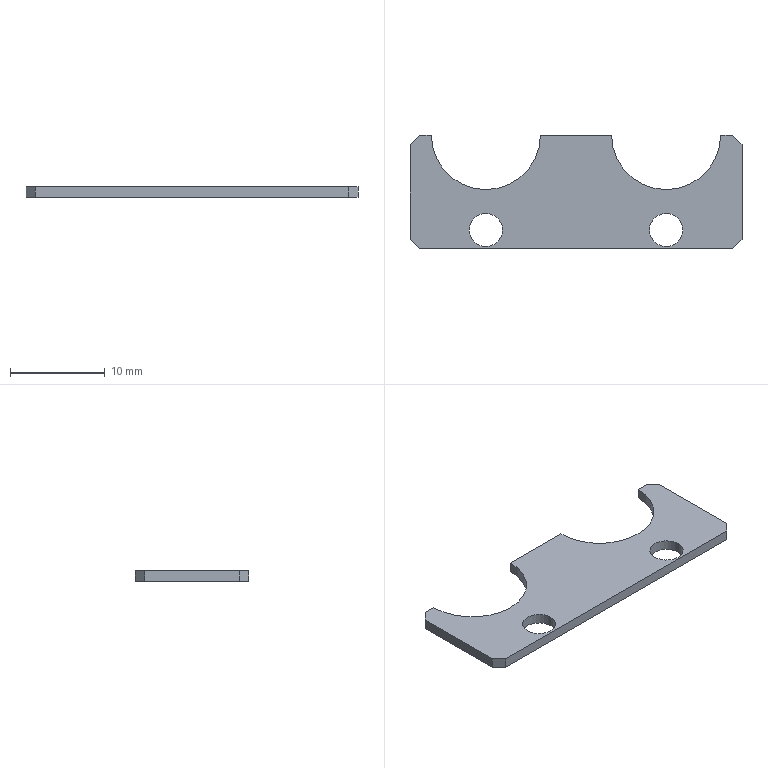Part | STEP file | 11-FG-SB00611 | 1 solid | 18 faces | box 35 x 12 x 1.1 mm | volume 324.378 mm3 | plane 12 | cylinder 6 | commonest cylinder face diameters 3.5 x4 11.5 x2
STEP:
#1=CARTESIAN_POINT('',(7.75,-4.,0.));
#2=VERTEX_POINT('',#1);
#3=CARTESIAN_POINT('',(11.25,-4.,0.));
#4=VERTEX_POINT('',#3);
#5=CARTESIAN_POINT('',(9.5,-4.,0.));
#6=DIRECTION('',(0.,0.,1.));
#7=DIRECTION('',(-1.,0.,0.));
#8=AXIS2_PLACEMENT_3D('',#5,#6,#7);
#9=CIRCLE('',#8,1.75);
#10=EDGE_CURVE('',#2,#4,#9,.T.);
#11=ORIENTED_EDGE('',*,*,#10,.F.);
#12=CARTESIAN_POINT('',(7.75,-4.,1.1));
#13=VERTEX_POINT('',#12);
#14=CARTESIAN_POINT('',(7.75,-4.,0.));
#15=DIRECTION('',(0.,0.,1.));
#16=VECTOR('',#15,1000.);
#17=LINE('',#14,#16);
#18=EDGE_CURVE('',#2,#13,#17,.T.);
#19=ORIENTED_EDGE('',*,*,#18,.T.);
#20=CARTESIAN_POINT('',(11.25,-4.,1.1));
#21=VERTEX_POINT('',#20);
#22=CARTESIAN_POINT('',(9.5,-4.,1.1));
#23=DIRECTION('',(0.,0.,1.));
#24=DIRECTION('',(-1.,0.,0.));
#25=AXIS2_PLACEMENT_3D('',#22,#23,#24);
#26=CIRCLE('',#25,1.75);
#27=EDGE_CURVE('',#13,#21,#26,.T.);
#28=ORIENTED_EDGE('',*,*,#27,.T.);
#29=CARTESIAN_POINT('',(11.25,-4.,0.));
#30=DIRECTION('',(0.,0.,1.));
#31=VECTOR('',#30,1000.);
#32=LINE('',#29,#31);
#33=EDGE_CURVE('',#4,#21,#32,.T.);
#34=ORIENTED_EDGE('',*,*,#33,.F.);
#35=EDGE_LOOP('',(#11,#19,#28,#34));
#36=FACE_OUTER_BOUND('',#35,.T.);
#37=CARTESIAN_POINT('',(9.5,-4.,0.));
#38=DIRECTION('',(0.,0.,1.));
#39=DIRECTION('',(1.,0.,0.));
#40=AXIS2_PLACEMENT_3D('',#37,#38,#39);
#41=CYLINDRICAL_SURFACE('',#40,1.75);
#42=ADVANCED_FACE('',(#36),#41,.F.);
#43=CARTESIAN_POINT('',(-11.25,-4.,0.));
#44=VERTEX_POINT('',#43);
#45=CARTESIAN_POINT('',(-7.75,-4.,0.));
#46=VERTEX_POINT('',#45);
#47=CARTESIAN_POINT('',(-9.5,-4.,0.));
#48=DIRECTION('',(0.,0.,1.));
#49=DIRECTION('',(1.,0.,0.));
#50=AXIS2_PLACEMENT_3D('',#47,#48,#49);
#51=CIRCLE('',#50,1.75);
#52=EDGE_CURVE('',#44,#46,#51,.T.);
#53=ORIENTED_EDGE('',*,*,#52,.F.);
#54=CARTESIAN_POINT('',(-11.25,-4.,1.1));
#55=VERTEX_POINT('',#54);
#56=CARTESIAN_POINT('',(-11.25,-4.,0.));
#57=DIRECTION('',(0.,0.,1.));
#58=VECTOR('',#57,1000.);
#59=LINE('',#56,#58);
#60=EDGE_CURVE('',#44,#55,#59,.T.);
#61=ORIENTED_EDGE('',*,*,#60,.T.);
#62=CARTESIAN_POINT('',(-7.75,-4.,1.1));
#63=VERTEX_POINT('',#62);
#64=CARTESIAN_POINT('',(-9.5,-4.,1.1));
#65=DIRECTION('',(0.,0.,1.));
#66=DIRECTION('',(1.,0.,0.));
#67=AXIS2_PLACEMENT_3D('',#64,#65,#66);
#68=CIRCLE('',#67,1.75);
#69=EDGE_CURVE('',#55,#63,#68,.T.);
#70=ORIENTED_EDGE('',*,*,#69,.T.);
#71=CARTESIAN_POINT('',(-7.75,-4.,0.));
#72=DIRECTION('',(0.,0.,1.));
#73=VECTOR('',#72,1000.);
#74=LINE('',#71,#73);
#75=EDGE_CURVE('',#46,#63,#74,.T.);
#76=ORIENTED_EDGE('',*,*,#75,.F.);
#77=EDGE_LOOP('',(#53,#61,#70,#76));
#78=FACE_OUTER_BOUND('',#77,.T.);
#79=CARTESIAN_POINT('',(-9.5,-4.,0.));
#80=DIRECTION('',(0.,0.,1.));
#81=DIRECTION('',(1.,0.,0.));
#82=AXIS2_PLACEMENT_3D('',#79,#80,#81);
#83=CYLINDRICAL_SURFACE('',#82,1.75);
#84=ADVANCED_FACE('',(#78),#83,.F.);
#85=CARTESIAN_POINT('',(16.5,6.,1.1));
#86=VERTEX_POINT('',#85);
#87=CARTESIAN_POINT('',(15.25,6.,1.1));
#88=VERTEX_POINT('',#87);
#89=CARTESIAN_POINT('',(-17.5,6.,1.1));
#90=DIRECTION('',(-1.,0.,0.));
#91=VECTOR('',#90,1000.);
#92=LINE('',#89,#91);
#93=EDGE_CURVE('',#86,#88,#92,.T.);
#94=ORIENTED_EDGE('',*,*,#93,.F.);
#95=CARTESIAN_POINT('',(16.5,6.,0.));
#96=VERTEX_POINT('',#95);
#97=CARTESIAN_POINT('',(16.5,6.,1.1));
#98=DIRECTION('',(0.,0.,-1.));
#99=VECTOR('',#98,1000.);
#100=LINE('',#97,#99);
#101=EDGE_CURVE('',#86,#96,#100,.T.);
#102=ORIENTED_EDGE('',*,*,#101,.T.);
#103=CARTESIAN_POINT('',(15.25,6.,0.));
#104=VERTEX_POINT('',#103);
#105=CARTESIAN_POINT('',(-17.5,6.,0.));
#106=DIRECTION('',(-1.,0.,0.));
#107=VECTOR('',#106,1000.);
#108=LINE('',#105,#107);
#109=EDGE_CURVE('',#96,#104,#108,.T.);
#110=ORIENTED_EDGE('',*,*,#109,.T.);
#111=CARTESIAN_POINT('',(15.25,6.,0.));
#112=DIRECTION('',(0.,0.,1.));
#113=VECTOR('',#112,1000.);
#114=LINE('',#111,#113);
#115=EDGE_CURVE('',#104,#88,#114,.T.);
#116=ORIENTED_EDGE('',*,*,#115,.T.);
#117=EDGE_LOOP('',(#94,#102,#110,#116));
#118=FACE_OUTER_BOUND('',#117,.T.);
#119=CARTESIAN_POINT('',(-17.5,6.,1.1));
#120=DIRECTION('',(0.,-1.,0.));
#121=DIRECTION('',(0.,0.,-1.));
#122=AXIS2_PLACEMENT_3D('',#119,#120,#121);
#123=PLANE('',#122);
#124=ADVANCED_FACE('',(#118),#123,.F.);
#125=CARTESIAN_POINT('',(3.75,6.,1.1));
#126=VERTEX_POINT('',#125);
#127=CARTESIAN_POINT('',(-3.75,6.,1.1));
#128=VERTEX_POINT('',#127);
#129=CARTESIAN_POINT('',(-17.5,6.,1.1));
#130=DIRECTION('',(-1.,0.,0.));
#131=VECTOR('',#130,1000.);
#132=LINE('',#129,#131);
#133=EDGE_CURVE('',#126,#128,#132,.T.);
#134=ORIENTED_EDGE('',*,*,#133,.F.);
#135=CARTESIAN_POINT('',(3.75,6.,0.));
#136=VERTEX_POINT('',#135);
#137=CARTESIAN_POINT('',(3.75,6.,0.));
#138=DIRECTION('',(0.,0.,-1.));
#139=VECTOR('',#138,1000.);
#140=LINE('',#137,#139);
#141=EDGE_CURVE('',#126,#136,#140,.T.);
#142=ORIENTED_EDGE('',*,*,#141,.T.);
#143=CARTESIAN_POINT('',(-3.75,6.,0.));
#144=VERTEX_POINT('',#143);
#145=CARTESIAN_POINT('',(-17.5,6.,0.));
#146=DIRECTION('',(-1.,0.,0.));
#147=VECTOR('',#146,1000.);
#148=LINE('',#145,#147);
#149=EDGE_CURVE('',#136,#144,#148,.T.);
#150=ORIENTED_EDGE('',*,*,#149,.T.);
#151=CARTESIAN_POINT('',(-3.75,6.,0.));
#152=DIRECTION('',(0.,0.,1.));
#153=VECTOR('',#152,1000.);
#154=LINE('',#151,#153);
#155=EDGE_CURVE('',#144,#128,#154,.T.);
#156=ORIENTED_EDGE('',*,*,#155,.T.);
#157=EDGE_LOOP('',(#134,#142,#150,#156));
#158=FACE_OUTER_BOUND('',#157,.T.);
#159=CARTESIAN_POINT('',(-17.5,6.,1.1));
#160=DIRECTION('',(0.,-1.,0.));
#161=DIRECTION('',(0.,0.,-1.));
#162=AXIS2_PLACEMENT_3D('',#159,#160,#161);
#163=PLANE('',#162);
#164=ADVANCED_FACE('',(#158),#163,.F.);
#165=CARTESIAN_POINT('',(17.5,-5.,0.));
#166=VERTEX_POINT('',#165);
#167=CARTESIAN_POINT('',(17.5,5.,0.));
#168=VERTEX_POINT('',#167);
#169=CARTESIAN_POINT('',(17.5,6.,0.));
#170=DIRECTION('',(0.,1.,0.));
#171=VECTOR('',#170,1000.);
#172=LINE('',#169,#171);
#173=EDGE_CURVE('',#166,#168,#172,.T.);
#174=ORIENTED_EDGE('',*,*,#173,.T.);
#175=CARTESIAN_POINT('',(17.5,5.,1.1));
#176=VERTEX_POINT('',#175);
#177=CARTESIAN_POINT('',(17.5,5.,1.1));
#178=DIRECTION('',(0.,0.,1.));
#179=VECTOR('',#178,1000.);
#180=LINE('',#177,#179);
#181=EDGE_CURVE('',#168,#176,#180,.T.);
#182=ORIENTED_EDGE('',*,*,#181,.T.);
#183=CARTESIAN_POINT('',(17.5,-5.,1.1));
#184=VERTEX_POINT('',#183);
#185=CARTESIAN_POINT('',(17.5,6.,1.1));
#186=DIRECTION('',(0.,1.,0.));
#187=VECTOR('',#186,1000.);
#188=LINE('',#185,#187);
#189=EDGE_CURVE('',#184,#176,#188,.T.);
#190=ORIENTED_EDGE('',*,*,#189,.F.);
#191=CARTESIAN_POINT('',(17.5,-5.,1.1));
#192=DIRECTION('',(0.,0.,-1.));
#193=VECTOR('',#192,1000.);
#194=LINE('',#191,#193);
#195=EDGE_CURVE('',#184,#166,#194,.T.);
#196=ORIENTED_EDGE('',*,*,#195,.T.);
#197=EDGE_LOOP('',(#174,#182,#190,#196));
#198=FACE_OUTER_BOUND('',#197,.T.);
#199=CARTESIAN_POINT('',(17.5,6.,1.1));
#200=DIRECTION('',(-1.,0.,0.));
#201=DIRECTION('',(0.,0.,1.));
#202=AXIS2_PLACEMENT_3D('',#199,#200,#201);
#203=PLANE('',#202);
#204=ADVANCED_FACE('',(#198),#203,.F.);
#205=CARTESIAN_POINT('',(-15.25,6.,0.));
#206=VERTEX_POINT('',#205);
#207=CARTESIAN_POINT('',(-16.5,6.,0.));
#208=VERTEX_POINT('',#207);
#209=CARTESIAN_POINT('',(-17.5,6.,0.));
#210=DIRECTION('',(-1.,0.,0.));
#211=VECTOR('',#210,1000.);
#212=LINE('',#209,#211);
#213=EDGE_CURVE('',#206,#208,#212,.T.);
#214=ORIENTED_EDGE('',*,*,#213,.T.);
#215=CARTESIAN_POINT('',(-16.5,6.,1.1));
#216=VERTEX_POINT('',#215);
#217=CARTESIAN_POINT('',(-16.5,6.,1.1));
#218=DIRECTION('',(0.,0.,1.));
#219=VECTOR('',#218,1000.);
#220=LINE('',#217,#219);
#221=EDGE_CURVE('',#208,#216,#220,.T.);
#222=ORIENTED_EDGE('',*,*,#221,.T.);
#223=CARTESIAN_POINT('',(-15.25,6.,1.1));
#224=VERTEX_POINT('',#223);
#225=CARTESIAN_POINT('',(-17.5,6.,1.1));
#226=DIRECTION('',(-1.,0.,0.));
#227=VECTOR('',#226,1000.);
#228=LINE('',#225,#227);
#229=EDGE_CURVE('',#224,#216,#228,.T.);
#230=ORIENTED_EDGE('',*,*,#229,.F.);
#231=CARTESIAN_POINT('',(-15.25,6.,0.));
#232=DIRECTION('',(0.,0.,-1.));
#233=VECTOR('',#232,1000.);
#234=LINE('',#231,#233);
#235=EDGE_CURVE('',#224,#206,#234,.T.);
#236=ORIENTED_EDGE('',*,*,#235,.T.);
#237=EDGE_LOOP('',(#214,#222,#230,#236));
#238=FACE_OUTER_BOUND('',#237,.T.);
#239=CARTESIAN_POINT('',(-17.5,6.,1.1));
#240=DIRECTION('',(0.,-1.,0.));
#241=DIRECTION('',(0.,0.,-1.));
#242=AXIS2_PLACEMENT_3D('',#239,#240,#241);
#243=PLANE('',#242);
#244=ADVANCED_FACE('',(#238),#243,.F.);
#245=CARTESIAN_POINT('',(-17.5,5.,1.1));
#246=VERTEX_POINT('',#245);
#247=CARTESIAN_POINT('',(-17.5,-5.,1.1));
#248=VERTEX_POINT('',#247);
#249=CARTESIAN_POINT('',(-17.5,6.,1.1));
#250=DIRECTION('',(0.,-1.,0.));
#251=VECTOR('',#250,1000.);
#252=LINE('',#249,#251);
#253=EDGE_CURVE('',#246,#248,#252,.T.);
#254=ORIENTED_EDGE('',*,*,#253,.F.);
#255=CARTESIAN_POINT('',(-17.5,5.,0.));
#256=VERTEX_POINT('',#255);
#257=CARTESIAN_POINT('',(-17.5,5.,1.1));
#258=DIRECTION('',(0.,0.,-1.));
#259=VECTOR('',#258,1000.);
#260=LINE('',#257,#259);
#261=EDGE_CURVE('',#246,#256,#260,.T.);
#262=ORIENTED_EDGE('',*,*,#261,.T.);
#263=CARTESIAN_POINT('',(-17.5,-5.,0.));
#264=VERTEX_POINT('',#263);
#265=CARTESIAN_POINT('',(-17.5,6.,0.));
#266=DIRECTION('',(0.,-1.,0.));
#267=VECTOR('',#266,1000.);
#268=LINE('',#265,#267);
#269=EDGE_CURVE('',#256,#264,#268,.T.);
#270=ORIENTED_EDGE('',*,*,#269,.T.);
#271=CARTESIAN_POINT('',(-17.5,-5.,1.1));
#272=DIRECTION('',(0.,0.,1.));
#273=VECTOR('',#272,1000.);
#274=LINE('',#271,#273);
#275=EDGE_CURVE('',#264,#248,#274,.T.);
#276=ORIENTED_EDGE('',*,*,#275,.T.);
#277=EDGE_LOOP('',(#254,#262,#270,#276));
#278=FACE_OUTER_BOUND('',#277,.T.);
#279=CARTESIAN_POINT('',(-17.5,6.,1.1));
#280=DIRECTION('',(1.,0.,0.));
#281=DIRECTION('',(0.,1.,0.));
#282=AXIS2_PLACEMENT_3D('',#279,#280,#281);
#283=PLANE('',#282);
#284=ADVANCED_FACE('',(#278),#283,.F.);
#285=CARTESIAN_POINT('',(-16.5,-6.,1.1));
#286=VERTEX_POINT('',#285);
#287=CARTESIAN_POINT('',(16.5,-6.,1.1));
#288=VERTEX_POINT('',#287);
#289=CARTESIAN_POINT('',(-17.5,-6.,1.1));
#290=DIRECTION('',(1.,0.,0.));
#291=VECTOR('',#290,1000.);
#292=LINE('',#289,#291);
#293=EDGE_CURVE('',#286,#288,#292,.T.);
#294=ORIENTED_EDGE('',*,*,#293,.F.);
#295=CARTESIAN_POINT('',(-16.5,-6.,0.));
#296=VERTEX_POINT('',#295);
#297=CARTESIAN_POINT('',(-16.5,-6.,1.1));
#298=DIRECTION('',(0.,0.,-1.));
#299=VECTOR('',#298,1000.);
#300=LINE('',#297,#299);
#301=EDGE_CURVE('',#286,#296,#300,.T.);
#302=ORIENTED_EDGE('',*,*,#301,.T.);
#303=CARTESIAN_POINT('',(16.5,-6.,0.));
#304=VERTEX_POINT('',#303);
#305=CARTESIAN_POINT('',(-17.5,-6.,0.));
#306=DIRECTION('',(1.,0.,0.));
#307=VECTOR('',#306,1000.);
#308=LINE('',#305,#307);
#309=EDGE_CURVE('',#296,#304,#308,.T.);
#310=ORIENTED_EDGE('',*,*,#309,.T.);
#311=CARTESIAN_POINT('',(16.5,-6.,1.1));
#312=DIRECTION('',(0.,0.,1.));
#313=VECTOR('',#312,1000.);
#314=LINE('',#311,#313);
#315=EDGE_CURVE('',#304,#288,#314,.T.);
#316=ORIENTED_EDGE('',*,*,#315,.T.);
#317=EDGE_LOOP('',(#294,#302,#310,#316));
#318=FACE_OUTER_BOUND('',#317,.T.);
#319=CARTESIAN_POINT('',(-17.5,-6.,1.1));
#320=DIRECTION('',(0.,1.,0.));
#321=DIRECTION('',(0.,0.,1.));
#322=AXIS2_PLACEMENT_3D('',#319,#320,#321);
#323=PLANE('',#322);
#324=ADVANCED_FACE('',(#318),#323,.F.);
#325=CARTESIAN_POINT('',(9.5,-4.,1.1));
#326=DIRECTION('',(0.,0.,1.));
#327=DIRECTION('',(-1.,0.,0.));
#328=AXIS2_PLACEMENT_3D('',#325,#326,#327);
#329=CIRCLE('',#328,1.75);
#330=EDGE_CURVE('',#21,#13,#329,.T.);
#331=ORIENTED_EDGE('',*,*,#330,.F.);
#332=ORIENTED_EDGE('',*,*,#27,.F.);
#333=EDGE_LOOP('',(#331,#332));
#334=FACE_BOUND('',#333,.T.);
#335=CARTESIAN_POINT('',(-9.5,-4.,1.1));
#336=DIRECTION('',(0.,0.,1.));
#337=DIRECTION('',(1.,0.,0.));
#338=AXIS2_PLACEMENT_3D('',#335,#336,#337);
#339=CIRCLE('',#338,1.75);
#340=EDGE_CURVE('',#63,#55,#339,.T.);
#341=ORIENTED_EDGE('',*,*,#340,.F.);
#342=ORIENTED_EDGE('',*,*,#69,.F.);
#343=EDGE_LOOP('',(#341,#342));
#344=FACE_BOUND('',#343,.T.);
#345=ORIENTED_EDGE('',*,*,#189,.T.);
#346=CARTESIAN_POINT('',(11.25,11.25,1.1));
#347=DIRECTION('',(-0.7071,0.7071,0.));
#348=VECTOR('',#347,1000.);
#349=LINE('',#346,#348);
#350=EDGE_CURVE('',#176,#86,#349,.T.);
#351=ORIENTED_EDGE('',*,*,#350,.T.);
#352=ORIENTED_EDGE('',*,*,#93,.T.);
#353=CARTESIAN_POINT('',(9.5,6.,1.1));
#354=DIRECTION('',(0.,0.,1.));
#355=DIRECTION('',(-1.,0.,0.));
#356=AXIS2_PLACEMENT_3D('',#353,#354,#355);
#357=CIRCLE('',#356,5.75);
#358=EDGE_CURVE('',#126,#88,#357,.T.);
#359=ORIENTED_EDGE('',*,*,#358,.F.);
#360=ORIENTED_EDGE('',*,*,#133,.T.);
#361=CARTESIAN_POINT('',(-9.5,6.,1.1));
#362=DIRECTION('',(0.,0.,1.));
#363=DIRECTION('',(1.,0.,0.));
#364=AXIS2_PLACEMENT_3D('',#361,#362,#363);
#365=CIRCLE('',#364,5.75);
#366=EDGE_CURVE('',#224,#128,#365,.T.);
#367=ORIENTED_EDGE('',*,*,#366,.F.);
#368=ORIENTED_EDGE('',*,*,#229,.T.);
#369=CARTESIAN_POINT('',(-11.25,11.25,1.1));
#370=DIRECTION('',(-0.7071,-0.7071,0.));
#371=VECTOR('',#370,1000.);
#372=LINE('',#369,#371);
#373=EDGE_CURVE('',#216,#246,#372,.T.);
#374=ORIENTED_EDGE('',*,*,#373,.T.);
#375=ORIENTED_EDGE('',*,*,#253,.T.);
#376=CARTESIAN_POINT('',(-11.25,-11.25,1.1));
#377=DIRECTION('',(0.7071,-0.7071,0.));
#378=VECTOR('',#377,1000.);
#379=LINE('',#376,#378);
#380=EDGE_CURVE('',#248,#286,#379,.T.);
#381=ORIENTED_EDGE('',*,*,#380,.T.);
#382=ORIENTED_EDGE('',*,*,#293,.T.);
#383=CARTESIAN_POINT('',(11.25,-11.25,1.1));
#384=DIRECTION('',(0.7071,0.7071,0.));
#385=VECTOR('',#384,1000.);
#386=LINE('',#383,#385);
#387=EDGE_CURVE('',#288,#184,#386,.T.);
#388=ORIENTED_EDGE('',*,*,#387,.T.);
#389=EDGE_LOOP('',(#345,#351,#352,#359,#360,#367,#368,#374,#375,#381,#382,#388));
#390=FACE_OUTER_BOUND('',#389,.T.);
#391=CARTESIAN_POINT('',(0.,0.,1.1));
#392=DIRECTION('',(0.,0.,1.));
#393=DIRECTION('',(1.,0.,0.));
#394=AXIS2_PLACEMENT_3D('',#391,#392,#393);
#395=PLANE('',#394);
#396=ADVANCED_FACE('',(#334,#344,#390),#395,.T.);
#397=CARTESIAN_POINT('',(9.5,-4.,0.));
#398=DIRECTION('',(0.,0.,1.));
#399=DIRECTION('',(-1.,0.,0.));
#400=AXIS2_PLACEMENT_3D('',#397,#398,#399);
#401=CIRCLE('',#400,1.75);
#402=EDGE_CURVE('',#4,#2,#401,.T.);
#403=ORIENTED_EDGE('',*,*,#402,.T.);
#404=ORIENTED_EDGE('',*,*,#10,.T.);
#405=EDGE_LOOP('',(#403,#404));
#406=FACE_BOUND('',#405,.T.);
#407=CARTESIAN_POINT('',(-9.5,-4.,0.));
#408=DIRECTION('',(0.,0.,1.));
#409=DIRECTION('',(1.,0.,0.));
#410=AXIS2_PLACEMENT_3D('',#407,#408,#409);
#411=CIRCLE('',#410,1.75);
#412=EDGE_CURVE('',#46,#44,#411,.T.);
#413=ORIENTED_EDGE('',*,*,#412,.T.);
#414=ORIENTED_EDGE('',*,*,#52,.T.);
#415=EDGE_LOOP('',(#413,#414));
#416=FACE_BOUND('',#415,.T.);
#417=ORIENTED_EDGE('',*,*,#109,.F.);
#418=CARTESIAN_POINT('',(16.5,6.,0.));
#419=DIRECTION('',(0.7071,-0.7071,0.));
#420=VECTOR('',#419,1000.);
#421=LINE('',#418,#420);
#422=EDGE_CURVE('',#96,#168,#421,.T.);
#423=ORIENTED_EDGE('',*,*,#422,.T.);
#424=ORIENTED_EDGE('',*,*,#173,.F.);
#425=CARTESIAN_POINT('',(17.5,-5.,0.));
#426=DIRECTION('',(-0.7071,-0.7071,0.));
#427=VECTOR('',#426,1000.);
#428=LINE('',#425,#427);
#429=EDGE_CURVE('',#166,#304,#428,.T.);
#430=ORIENTED_EDGE('',*,*,#429,.T.);
#431=ORIENTED_EDGE('',*,*,#309,.F.);
#432=CARTESIAN_POINT('',(-16.5,-6.,0.));
#433=DIRECTION('',(-0.7071,0.7071,0.));
#434=VECTOR('',#433,1000.);
#435=LINE('',#432,#434);
#436=EDGE_CURVE('',#296,#264,#435,.T.);
#437=ORIENTED_EDGE('',*,*,#436,.T.);
#438=ORIENTED_EDGE('',*,*,#269,.F.);
#439=CARTESIAN_POINT('',(-17.5,5.,0.));
#440=DIRECTION('',(0.7071,0.7071,0.));
#441=VECTOR('',#440,1000.);
#442=LINE('',#439,#441);
#443=EDGE_CURVE('',#256,#208,#442,.T.);
#444=ORIENTED_EDGE('',*,*,#443,.T.);
#445=ORIENTED_EDGE('',*,*,#213,.F.);
#446=CARTESIAN_POINT('',(-9.5,6.,0.));
#447=DIRECTION('',(0.,0.,1.));
#448=DIRECTION('',(1.,0.,0.));
#449=AXIS2_PLACEMENT_3D('',#446,#447,#448);
#450=CIRCLE('',#449,5.75);
#451=EDGE_CURVE('',#206,#144,#450,.T.);
#452=ORIENTED_EDGE('',*,*,#451,.T.);
#453=ORIENTED_EDGE('',*,*,#149,.F.);
#454=CARTESIAN_POINT('',(9.5,6.,0.));
#455=DIRECTION('',(0.,0.,1.));
#456=DIRECTION('',(-1.,0.,0.));
#457=AXIS2_PLACEMENT_3D('',#454,#455,#456);
#458=CIRCLE('',#457,5.75);
#459=EDGE_CURVE('',#136,#104,#458,.T.);
#460=ORIENTED_EDGE('',*,*,#459,.T.);
#461=EDGE_LOOP('',(#417,#423,#424,#430,#431,#437,#438,#444,#445,#452,#453,#460));
#462=FACE_OUTER_BOUND('',#461,.T.);
#463=CARTESIAN_POINT('',(0.,0.,0.));
#464=DIRECTION('',(0.,0.,1.));
#465=DIRECTION('',(1.,0.,0.));
#466=AXIS2_PLACEMENT_3D('',#463,#464,#465);
#467=PLANE('',#466);
#468=ADVANCED_FACE('',(#406,#416,#462),#467,.F.);
#469=ORIENTED_EDGE('',*,*,#451,.F.);
#470=ORIENTED_EDGE('',*,*,#235,.F.);
#471=ORIENTED_EDGE('',*,*,#366,.T.);
#472=ORIENTED_EDGE('',*,*,#155,.F.);
#473=EDGE_LOOP('',(#469,#470,#471,#472));
#474=FACE_OUTER_BOUND('',#473,.T.);
#475=CARTESIAN_POINT('',(-9.5,6.,0.));
#476=DIRECTION('',(0.,0.,1.));
#477=DIRECTION('',(1.,0.,0.));
#478=AXIS2_PLACEMENT_3D('',#475,#476,#477);
#479=CYLINDRICAL_SURFACE('',#478,5.75);
#480=ADVANCED_FACE('',(#474),#479,.F.);
#481=ORIENTED_EDGE('',*,*,#459,.F.);
#482=ORIENTED_EDGE('',*,*,#141,.F.);
#483=ORIENTED_EDGE('',*,*,#358,.T.);
#484=ORIENTED_EDGE('',*,*,#115,.F.);
#485=EDGE_LOOP('',(#481,#482,#483,#484));
#486=FACE_OUTER_BOUND('',#485,.T.);
#487=CARTESIAN_POINT('',(9.5,6.,0.));
#488=DIRECTION('',(0.,0.,1.));
#489=DIRECTION('',(1.,0.,0.));
#490=AXIS2_PLACEMENT_3D('',#487,#488,#489);
#491=CYLINDRICAL_SURFACE('',#490,5.75);
#492=ADVANCED_FACE('',(#486),#491,.F.);
#493=ORIENTED_EDGE('',*,*,#60,.F.);
#494=ORIENTED_EDGE('',*,*,#412,.F.);
#495=ORIENTED_EDGE('',*,*,#75,.T.);
#496=ORIENTED_EDGE('',*,*,#340,.T.);
#497=EDGE_LOOP('',(#493,#494,#495,#496));
#498=FACE_OUTER_BOUND('',#497,.T.);
#499=CARTESIAN_POINT('',(-9.5,-4.,0.));
#500=DIRECTION('',(0.,0.,1.));
#501=DIRECTION('',(1.,0.,0.));
#502=AXIS2_PLACEMENT_3D('',#499,#500,#501);
#503=CYLINDRICAL_SURFACE('',#502,1.75);
#504=ADVANCED_FACE('',(#498),#503,.F.);
#505=ORIENTED_EDGE('',*,*,#18,.F.);
#506=ORIENTED_EDGE('',*,*,#402,.F.);
#507=ORIENTED_EDGE('',*,*,#33,.T.);
#508=ORIENTED_EDGE('',*,*,#330,.T.);
#509=EDGE_LOOP('',(#505,#506,#507,#508));
#510=FACE_OUTER_BOUND('',#509,.T.);
#511=CARTESIAN_POINT('',(9.5,-4.,0.));
#512=DIRECTION('',(0.,0.,1.));
#513=DIRECTION('',(1.,0.,0.));
#514=AXIS2_PLACEMENT_3D('',#511,#512,#513);
#515=CYLINDRICAL_SURFACE('',#514,1.75);
#516=ADVANCED_FACE('',(#510),#515,.F.);
#517=ORIENTED_EDGE('',*,*,#350,.F.);
#518=ORIENTED_EDGE('',*,*,#181,.F.);
#519=ORIENTED_EDGE('',*,*,#422,.F.);
#520=ORIENTED_EDGE('',*,*,#101,.F.);
#521=EDGE_LOOP('',(#517,#518,#519,#520));
#522=FACE_OUTER_BOUND('',#521,.T.);
#523=CARTESIAN_POINT('',(16.5,6.,1.1));
#524=DIRECTION('',(-0.7071,-0.7071,0.));
#525=DIRECTION('',(0.,0.,-1.));
#526=AXIS2_PLACEMENT_3D('',#523,#524,#525);
#527=PLANE('',#526);
#528=ADVANCED_FACE('',(#522),#527,.F.);
#529=ORIENTED_EDGE('',*,*,#373,.F.);
#530=ORIENTED_EDGE('',*,*,#221,.F.);
#531=ORIENTED_EDGE('',*,*,#443,.F.);
#532=ORIENTED_EDGE('',*,*,#261,.F.);
#533=EDGE_LOOP('',(#529,#530,#531,#532));
#534=FACE_OUTER_BOUND('',#533,.T.);
#535=CARTESIAN_POINT('',(-17.5,5.,1.1));
#536=DIRECTION('',(0.7071,-0.7071,0.));
#537=DIRECTION('',(0.,0.,-1.));
#538=AXIS2_PLACEMENT_3D('',#535,#536,#537);
#539=PLANE('',#538);
#540=ADVANCED_FACE('',(#534),#539,.F.);
#541=ORIENTED_EDGE('',*,*,#380,.F.);
#542=ORIENTED_EDGE('',*,*,#275,.F.);
#543=ORIENTED_EDGE('',*,*,#436,.F.);
#544=ORIENTED_EDGE('',*,*,#301,.F.);
#545=EDGE_LOOP('',(#541,#542,#543,#544));
#546=FACE_OUTER_BOUND('',#545,.T.);
#547=CARTESIAN_POINT('',(-16.5,-6.,1.1));
#548=DIRECTION('',(0.7071,0.7071,0.));
#549=DIRECTION('',(0.,0.,-1.));
#550=AXIS2_PLACEMENT_3D('',#547,#548,#549);
#551=PLANE('',#550);
#552=ADVANCED_FACE('',(#546),#551,.F.);
#553=ORIENTED_EDGE('',*,*,#387,.F.);
#554=ORIENTED_EDGE('',*,*,#315,.F.);
#555=ORIENTED_EDGE('',*,*,#429,.F.);
#556=ORIENTED_EDGE('',*,*,#195,.F.);
#557=EDGE_LOOP('',(#553,#554,#555,#556));
#558=FACE_OUTER_BOUND('',#557,.T.);
#559=CARTESIAN_POINT('',(17.5,-5.,1.1));
#560=DIRECTION('',(-0.7071,0.7071,0.));
#561=DIRECTION('',(0.,0.,-1.));
#562=AXIS2_PLACEMENT_3D('',#559,#560,#561);
#563=PLANE('',#562);
#564=ADVANCED_FACE('',(#558),#563,.F.);
#565=CLOSED_SHELL('',(#42,#84,#124,#164,#204,#244,#284,#324,#396,#468,#480,#492,#504,#516,#528,#540,#552,#564));
#566=MANIFOLD_SOLID_BREP('',#565);
#567=CARTESIAN_POINT('',(0.,0.,0.));
#568=DIRECTION('',(0.,0.,1.));
#569=DIRECTION('',(1.,0.,0.));
#570=AXIS2_PLACEMENT_3D('',#567,#568,#569);
#571=(LENGTH_UNIT()NAMED_UNIT(*)SI_UNIT(.MILLI.,.METRE.));
#572=UNCERTAINTY_MEASURE_WITH_UNIT(LENGTH_MEASURE(0.00001),#571,'','');
#573=(NAMED_UNIT(*)PLANE_ANGLE_UNIT()SI_UNIT($,.RADIAN.));
#574=(NAMED_UNIT(*)SI_UNIT($,.STERADIAN.)SOLID_ANGLE_UNIT());
#575=(GEOMETRIC_REPRESENTATION_CONTEXT(3)GLOBAL_UNCERTAINTY_ASSIGNED_CONTEXT((#572))GLOBAL_UNIT_ASSIGNED_CONTEXT((#571,#573,#574))REPRESENTATION_CONTEXT('',''));
#576=ADVANCED_BREP_SHAPE_REPRESENTATION('',(#566,#570),#575);